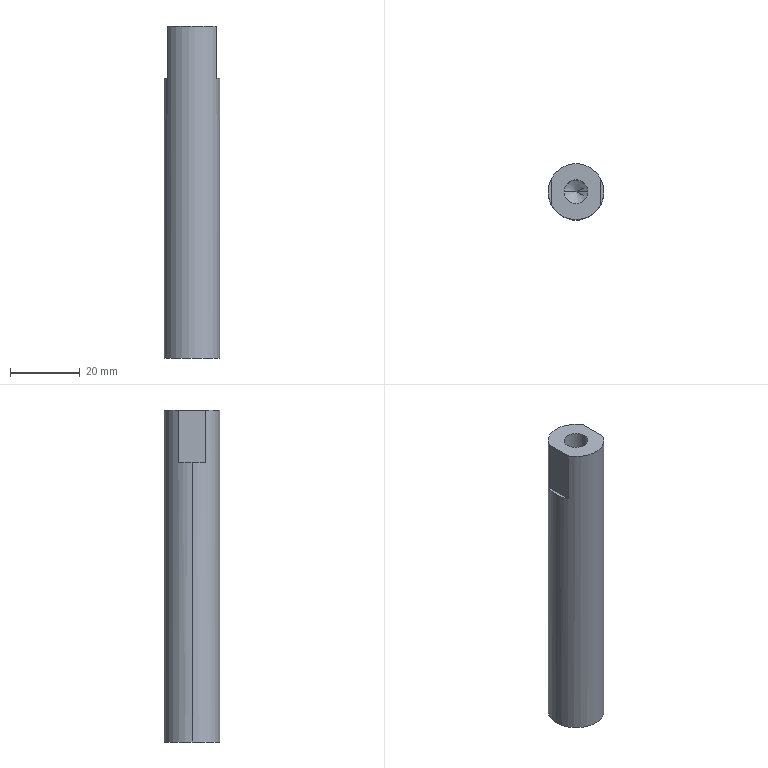Part | STEP file | 1 solid | 12 faces | box 16 x 16 x 95 mm | volume 18202 mm3 | plane 6 | cylinder 4 | cone 2 | commonest cylinder face diameters 6.8 x2 16 x2
STEP:
#1=CARTESIAN_POINT('',(-3.4,0.,180.25));
#2=VERTEX_POINT('',#1);
#3=CARTESIAN_POINT('',(3.4,0.,180.25));
#4=VERTEX_POINT('',#3);
#5=CARTESIAN_POINT('',(0.,0.,180.25));
#6=DIRECTION('',(0.,0.,1.));
#7=DIRECTION('',(1.,0.,0.));
#8=AXIS2_PLACEMENT_3D('',#5,#6,#7);
#9=CIRCLE('',#8,3.4);
#10=EDGE_CURVE('',#2,#4,#9,.T.);
#11=ORIENTED_EDGE('',*,*,#10,.F.);
#12=CARTESIAN_POINT('',(-3.4,0.,200.));
#13=VERTEX_POINT('',#12);
#14=CARTESIAN_POINT('',(-3.4,0.,200.));
#15=DIRECTION('',(0.,0.,1.));
#16=VECTOR('',#15,1000.);
#17=LINE('',#14,#16);
#18=EDGE_CURVE('',#2,#13,#17,.T.);
#19=ORIENTED_EDGE('',*,*,#18,.T.);
#20=CARTESIAN_POINT('',(3.4,0.,200.));
#21=VERTEX_POINT('',#20);
#22=CARTESIAN_POINT('',(0.,0.,200.));
#23=DIRECTION('',(0.,0.,1.));
#24=DIRECTION('',(1.,0.,0.));
#25=AXIS2_PLACEMENT_3D('',#22,#23,#24);
#26=CIRCLE('',#25,3.4);
#27=EDGE_CURVE('',#13,#21,#26,.T.);
#28=ORIENTED_EDGE('',*,*,#27,.T.);
#29=CARTESIAN_POINT('',(3.4,0.,200.));
#30=DIRECTION('',(0.,0.,1.));
#31=VECTOR('',#30,1000.);
#32=LINE('',#29,#31);
#33=EDGE_CURVE('',#4,#21,#32,.T.);
#34=ORIENTED_EDGE('',*,*,#33,.F.);
#35=EDGE_LOOP('',(#11,#19,#28,#34));
#36=FACE_OUTER_BOUND('',#35,.T.);
#37=CARTESIAN_POINT('',(0.,0.,200.));
#38=DIRECTION('',(0.,0.,1.));
#39=DIRECTION('',(1.,0.,0.));
#40=AXIS2_PLACEMENT_3D('',#37,#38,#39);
#41=CYLINDRICAL_SURFACE('',#40,3.4);
#42=ADVANCED_FACE('',(#36),#41,.F.);
#43=CARTESIAN_POINT('',(0.,0.,178.207));
#44=VERTEX_POINT('',#43);
#45=CARTESIAN_POINT('',(3.4,0.,180.25));
#46=DIRECTION('',(0.8572,0.,0.515));
#47=VECTOR('',#46,1000.);
#48=LINE('',#45,#47);
#49=EDGE_CURVE('',#44,#4,#48,.T.);
#50=ORIENTED_EDGE('',*,*,#49,.F.);
#51=CARTESIAN_POINT('',(-3.4,0.,180.25));
#52=DIRECTION('',(-0.8572,0.,0.515));
#53=VECTOR('',#52,1000.);
#54=LINE('',#51,#53);
#55=EDGE_CURVE('',#44,#2,#54,.T.);
#56=ORIENTED_EDGE('',*,*,#55,.T.);
#57=ORIENTED_EDGE('',*,*,#10,.T.);
#58=EDGE_LOOP('',(#50,#56,#57));
#59=FACE_OUTER_BOUND('',#58,.T.);
#60=CARTESIAN_POINT('',(0.,0.,180.25));
#61=DIRECTION('',(0.,0.,1.));
#62=DIRECTION('',(1.,0.,0.));
#63=AXIS2_PLACEMENT_3D('',#60,#61,#62);
#64=CONICAL_SURFACE('',#63,3.4,1.03);
#65=ADVANCED_FACE('',(#59),#64,.F.);
#66=CARTESIAN_POINT('',(-8.,0.,105.));
#67=VERTEX_POINT('',#66);
#68=CARTESIAN_POINT('',(8.,0.,105.));
#69=VERTEX_POINT('',#68);
#70=CARTESIAN_POINT('',(0.,0.,105.));
#71=DIRECTION('',(0.,0.,-1.));
#72=DIRECTION('',(-1.,0.,0.));
#73=AXIS2_PLACEMENT_3D('',#70,#71,#72);
#74=CIRCLE('',#73,8.);
#75=EDGE_CURVE('',#67,#69,#74,.T.);
#76=ORIENTED_EDGE('',*,*,#75,.F.);
#77=CARTESIAN_POINT('',(-8.,0.,185.));
#78=VERTEX_POINT('',#77);
#79=CARTESIAN_POINT('',(-8.,0.,-128.284));
#80=DIRECTION('',(0.,0.,1.));
#81=VECTOR('',#80,1000.);
#82=LINE('',#79,#81);
#83=EDGE_CURVE('',#67,#78,#82,.T.);
#84=ORIENTED_EDGE('',*,*,#83,.T.);
#85=CARTESIAN_POINT('',(-7.,3.873,185.));
#86=VERTEX_POINT('',#85);
#87=CARTESIAN_POINT('',(0.,0.,185.));
#88=DIRECTION('',(0.,0.,-1.));
#89=DIRECTION('',(1.,0.,0.));
#90=AXIS2_PLACEMENT_3D('',#87,#88,#89);
#91=CIRCLE('',#90,8.);
#92=EDGE_CURVE('',#78,#86,#91,.T.);
#93=ORIENTED_EDGE('',*,*,#92,.T.);
#94=CARTESIAN_POINT('',(-7.,3.873,200.));
#95=VERTEX_POINT('',#94);
#96=CARTESIAN_POINT('',(-7.,3.873,-128.284));
#97=DIRECTION('',(0.,0.,-1.));
#98=VECTOR('',#97,1000.);
#99=LINE('',#96,#98);
#100=EDGE_CURVE('',#95,#86,#99,.T.);
#101=ORIENTED_EDGE('',*,*,#100,.F.);
#102=CARTESIAN_POINT('',(7.,3.873,200.));
#103=VERTEX_POINT('',#102);
#104=CARTESIAN_POINT('',(0.,0.,200.));
#105=DIRECTION('',(0.,0.,1.));
#106=DIRECTION('',(1.,0.,0.));
#107=AXIS2_PLACEMENT_3D('',#104,#105,#106);
#108=CIRCLE('',#107,8.);
#109=EDGE_CURVE('',#103,#95,#108,.T.);
#110=ORIENTED_EDGE('',*,*,#109,.F.);
#111=CARTESIAN_POINT('',(7.,3.873,185.));
#112=VERTEX_POINT('',#111);
#113=CARTESIAN_POINT('',(7.,3.873,-128.284));
#114=DIRECTION('',(0.,0.,1.));
#115=VECTOR('',#114,1000.);
#116=LINE('',#113,#115);
#117=EDGE_CURVE('',#112,#103,#116,.T.);
#118=ORIENTED_EDGE('',*,*,#117,.F.);
#119=CARTESIAN_POINT('',(8.,0.,185.));
#120=VERTEX_POINT('',#119);
#121=CARTESIAN_POINT('',(0.,0.,185.));
#122=DIRECTION('',(0.,0.,-1.));
#123=DIRECTION('',(1.,0.,0.));
#124=AXIS2_PLACEMENT_3D('',#121,#122,#123);
#125=CIRCLE('',#124,8.);
#126=EDGE_CURVE('',#112,#120,#125,.T.);
#127=ORIENTED_EDGE('',*,*,#126,.T.);
#128=CARTESIAN_POINT('',(8.,0.,-128.284));
#129=DIRECTION('',(0.,0.,1.));
#130=VECTOR('',#129,1000.);
#131=LINE('',#128,#130);
#132=EDGE_CURVE('',#69,#120,#131,.T.);
#133=ORIENTED_EDGE('',*,*,#132,.F.);
#134=EDGE_LOOP('',(#76,#84,#93,#101,#110,#118,#127,#133));
#135=FACE_OUTER_BOUND('',#134,.T.);
#136=CARTESIAN_POINT('',(0.,0.,-128.284));
#137=DIRECTION('',(0.,0.,1.));
#138=DIRECTION('',(1.,0.,0.));
#139=AXIS2_PLACEMENT_3D('',#136,#137,#138);
#140=CYLINDRICAL_SURFACE('',#139,8.);
#141=ADVANCED_FACE('',(#135),#140,.T.);
#142=ORIENTED_EDGE('',*,*,#83,.F.);
#143=CARTESIAN_POINT('',(0.,0.,105.));
#144=DIRECTION('',(0.,0.,-1.));
#145=DIRECTION('',(-1.,0.,0.));
#146=AXIS2_PLACEMENT_3D('',#143,#144,#145);
#147=CIRCLE('',#146,8.);
#148=EDGE_CURVE('',#69,#67,#147,.T.);
#149=ORIENTED_EDGE('',*,*,#148,.F.);
#150=ORIENTED_EDGE('',*,*,#132,.T.);
#151=CARTESIAN_POINT('',(7.,-3.873,185.));
#152=VERTEX_POINT('',#151);
#153=CARTESIAN_POINT('',(0.,0.,185.));
#154=DIRECTION('',(0.,0.,-1.));
#155=DIRECTION('',(1.,0.,0.));
#156=AXIS2_PLACEMENT_3D('',#153,#154,#155);
#157=CIRCLE('',#156,8.);
#158=EDGE_CURVE('',#120,#152,#157,.T.);
#159=ORIENTED_EDGE('',*,*,#158,.T.);
#160=CARTESIAN_POINT('',(7.,-3.873,200.));
#161=VERTEX_POINT('',#160);
#162=CARTESIAN_POINT('',(7.,-3.873,-128.284));
#163=DIRECTION('',(0.,0.,-1.));
#164=VECTOR('',#163,1000.);
#165=LINE('',#162,#164);
#166=EDGE_CURVE('',#161,#152,#165,.T.);
#167=ORIENTED_EDGE('',*,*,#166,.F.);
#168=CARTESIAN_POINT('',(-7.,-3.873,200.));
#169=VERTEX_POINT('',#168);
#170=CARTESIAN_POINT('',(0.,0.,200.));
#171=DIRECTION('',(0.,0.,1.));
#172=DIRECTION('',(1.,0.,0.));
#173=AXIS2_PLACEMENT_3D('',#170,#171,#172);
#174=CIRCLE('',#173,8.);
#175=EDGE_CURVE('',#169,#161,#174,.T.);
#176=ORIENTED_EDGE('',*,*,#175,.F.);
#177=CARTESIAN_POINT('',(-7.,-3.873,185.));
#178=VERTEX_POINT('',#177);
#179=CARTESIAN_POINT('',(-7.,-3.873,-128.284));
#180=DIRECTION('',(0.,0.,1.));
#181=VECTOR('',#180,1000.);
#182=LINE('',#179,#181);
#183=EDGE_CURVE('',#178,#169,#182,.T.);
#184=ORIENTED_EDGE('',*,*,#183,.F.);
#185=CARTESIAN_POINT('',(0.,0.,185.));
#186=DIRECTION('',(0.,0.,-1.));
#187=DIRECTION('',(1.,0.,0.));
#188=AXIS2_PLACEMENT_3D('',#185,#186,#187);
#189=CIRCLE('',#188,8.);
#190=EDGE_CURVE('',#178,#78,#189,.T.);
#191=ORIENTED_EDGE('',*,*,#190,.T.);
#192=EDGE_LOOP('',(#142,#149,#150,#159,#167,#176,#184,#191));
#193=FACE_OUTER_BOUND('',#192,.T.);
#194=CARTESIAN_POINT('',(0.,0.,-128.284));
#195=DIRECTION('',(0.,0.,1.));
#196=DIRECTION('',(1.,0.,0.));
#197=AXIS2_PLACEMENT_3D('',#194,#195,#196);
#198=CYLINDRICAL_SURFACE('',#197,8.);
#199=ADVANCED_FACE('',(#193),#198,.T.);
#200=CARTESIAN_POINT('',(-7.,0.,200.));
#201=DIRECTION('',(0.,1.,0.));
#202=VECTOR('',#201,1000.);
#203=LINE('',#200,#202);
#204=EDGE_CURVE('',#169,#95,#203,.T.);
#205=ORIENTED_EDGE('',*,*,#204,.F.);
#206=ORIENTED_EDGE('',*,*,#175,.T.);
#207=CARTESIAN_POINT('',(7.,0.,200.));
#208=DIRECTION('',(0.,-1.,0.));
#209=VECTOR('',#208,1000.);
#210=LINE('',#207,#209);
#211=EDGE_CURVE('',#103,#161,#210,.T.);
#212=ORIENTED_EDGE('',*,*,#211,.F.);
#213=ORIENTED_EDGE('',*,*,#109,.T.);
#214=EDGE_LOOP('',(#205,#206,#212,#213));
#215=FACE_OUTER_BOUND('',#214,.T.);
#216=CARTESIAN_POINT('',(0.,0.,200.));
#217=DIRECTION('',(0.,0.,1.));
#218=DIRECTION('',(1.,0.,0.));
#219=AXIS2_PLACEMENT_3D('',#216,#217,#218);
#220=CIRCLE('',#219,3.4);
#221=EDGE_CURVE('',#21,#13,#220,.T.);
#222=ORIENTED_EDGE('',*,*,#221,.F.);
#223=ORIENTED_EDGE('',*,*,#27,.F.);
#224=EDGE_LOOP('',(#222,#223));
#225=FACE_BOUND('',#224,.T.);
#226=CARTESIAN_POINT('',(0.,0.,200.));
#227=DIRECTION('',(0.,0.,1.));
#228=DIRECTION('',(1.,0.,0.));
#229=AXIS2_PLACEMENT_3D('',#226,#227,#228);
#230=PLANE('',#229);
#231=ADVANCED_FACE('',(#215,#225),#230,.T.);
#232=ORIENTED_EDGE('',*,*,#148,.T.);
#233=ORIENTED_EDGE('',*,*,#75,.T.);
#234=EDGE_LOOP('',(#232,#233));
#235=FACE_OUTER_BOUND('',#234,.T.);
#236=CARTESIAN_POINT('',(0.,0.,105.));
#237=DIRECTION('',(0.,0.,-1.));
#238=DIRECTION('',(0.,-1.,0.));
#239=AXIS2_PLACEMENT_3D('',#236,#237,#238);
#240=PLANE('',#239);
#241=ADVANCED_FACE('',(#235),#240,.T.);
#242=ORIENTED_EDGE('',*,*,#166,.T.);
#243=CARTESIAN_POINT('',(7.,10.406,185.));
#244=DIRECTION('',(0.,-1.,0.));
#245=VECTOR('',#244,1000.);
#246=LINE('',#243,#245);
#247=EDGE_CURVE('',#112,#152,#246,.T.);
#248=ORIENTED_EDGE('',*,*,#247,.F.);
#249=ORIENTED_EDGE('',*,*,#117,.T.);
#250=ORIENTED_EDGE('',*,*,#211,.T.);
#251=EDGE_LOOP('',(#242,#248,#249,#250));
#252=FACE_OUTER_BOUND('',#251,.T.);
#253=CARTESIAN_POINT('',(7.,10.406,185.));
#254=DIRECTION('',(-1.,0.,0.));
#255=DIRECTION('',(0.,1.,0.));
#256=AXIS2_PLACEMENT_3D('',#253,#254,#255);
#257=PLANE('',#256);
#258=ADVANCED_FACE('',(#252),#257,.F.);
#259=ORIENTED_EDGE('',*,*,#247,.T.);
#260=ORIENTED_EDGE('',*,*,#158,.F.);
#261=ORIENTED_EDGE('',*,*,#126,.F.);
#262=EDGE_LOOP('',(#259,#260,#261));
#263=FACE_OUTER_BOUND('',#262,.T.);
#264=CARTESIAN_POINT('',(0.,0.,185.));
#265=DIRECTION('',(0.,0.,1.));
#266=DIRECTION('',(1.,0.,0.));
#267=AXIS2_PLACEMENT_3D('',#264,#265,#266);
#268=PLANE('',#267);
#269=ADVANCED_FACE('',(#263),#268,.T.);
#270=ORIENTED_EDGE('',*,*,#100,.T.);
#271=CARTESIAN_POINT('',(-7.,11.987,185.));
#272=DIRECTION('',(0.,1.,0.));
#273=VECTOR('',#272,1000.);
#274=LINE('',#271,#273);
#275=EDGE_CURVE('',#178,#86,#274,.T.);
#276=ORIENTED_EDGE('',*,*,#275,.F.);
#277=ORIENTED_EDGE('',*,*,#183,.T.);
#278=ORIENTED_EDGE('',*,*,#204,.T.);
#279=EDGE_LOOP('',(#270,#276,#277,#278));
#280=FACE_OUTER_BOUND('',#279,.T.);
#281=CARTESIAN_POINT('',(-7.,11.987,185.));
#282=DIRECTION('',(1.,0.,0.));
#283=DIRECTION('',(0.,0.,1.));
#284=AXIS2_PLACEMENT_3D('',#281,#282,#283);
#285=PLANE('',#284);
#286=ADVANCED_FACE('',(#280),#285,.F.);
#287=ORIENTED_EDGE('',*,*,#275,.T.);
#288=ORIENTED_EDGE('',*,*,#92,.F.);
#289=ORIENTED_EDGE('',*,*,#190,.F.);
#290=EDGE_LOOP('',(#287,#288,#289));
#291=FACE_OUTER_BOUND('',#290,.T.);
#292=CARTESIAN_POINT('',(0.,0.,185.));
#293=DIRECTION('',(0.,0.,1.));
#294=DIRECTION('',(1.,0.,0.));
#295=AXIS2_PLACEMENT_3D('',#292,#293,#294);
#296=PLANE('',#295);
#297=ADVANCED_FACE('',(#291),#296,.T.);
#298=ORIENTED_EDGE('',*,*,#55,.F.);
#299=ORIENTED_EDGE('',*,*,#49,.T.);
#300=CARTESIAN_POINT('',(0.,0.,180.25));
#301=DIRECTION('',(0.,0.,1.));
#302=DIRECTION('',(1.,0.,0.));
#303=AXIS2_PLACEMENT_3D('',#300,#301,#302);
#304=CIRCLE('',#303,3.4);
#305=EDGE_CURVE('',#4,#2,#304,.T.);
#306=ORIENTED_EDGE('',*,*,#305,.T.);
#307=EDGE_LOOP('',(#298,#299,#306));
#308=FACE_OUTER_BOUND('',#307,.T.);
#309=CARTESIAN_POINT('',(0.,0.,180.25));
#310=DIRECTION('',(0.,0.,1.));
#311=DIRECTION('',(1.,0.,0.));
#312=AXIS2_PLACEMENT_3D('',#309,#310,#311);
#313=CONICAL_SURFACE('',#312,3.4,1.03);
#314=ADVANCED_FACE('',(#308),#313,.F.);
#315=ORIENTED_EDGE('',*,*,#18,.F.);
#316=ORIENTED_EDGE('',*,*,#305,.F.);
#317=ORIENTED_EDGE('',*,*,#33,.T.);
#318=ORIENTED_EDGE('',*,*,#221,.T.);
#319=EDGE_LOOP('',(#315,#316,#317,#318));
#320=FACE_OUTER_BOUND('',#319,.T.);
#321=CARTESIAN_POINT('',(0.,0.,200.));
#322=DIRECTION('',(0.,0.,1.));
#323=DIRECTION('',(1.,0.,0.));
#324=AXIS2_PLACEMENT_3D('',#321,#322,#323);
#325=CYLINDRICAL_SURFACE('',#324,3.4);
#326=ADVANCED_FACE('',(#320),#325,.F.);
#327=CLOSED_SHELL('',(#42,#65,#141,#199,#231,#241,#258,#269,#286,#297,#314,#326));
#328=MANIFOLD_SOLID_BREP('',#327);
#329=CARTESIAN_POINT('',(0.,0.,0.));
#330=DIRECTION('',(0.,0.,1.));
#331=DIRECTION('',(1.,0.,0.));
#332=AXIS2_PLACEMENT_3D('',#329,#330,#331);
#333=(LENGTH_UNIT()NAMED_UNIT(*)SI_UNIT(.MILLI.,.METRE.));
#334=UNCERTAINTY_MEASURE_WITH_UNIT(LENGTH_MEASURE(0.00001),#333,'','');
#335=(NAMED_UNIT(*)PLANE_ANGLE_UNIT()SI_UNIT($,.RADIAN.));
#336=(NAMED_UNIT(*)SI_UNIT($,.STERADIAN.)SOLID_ANGLE_UNIT());
#337=(GEOMETRIC_REPRESENTATION_CONTEXT(3)GLOBAL_UNCERTAINTY_ASSIGNED_CONTEXT((#334))GLOBAL_UNIT_ASSIGNED_CONTEXT((#333,#335,#336))REPRESENTATION_CONTEXT('',''));
#338=ADVANCED_BREP_SHAPE_REPRESENTATION('',(#328,#332),#337);